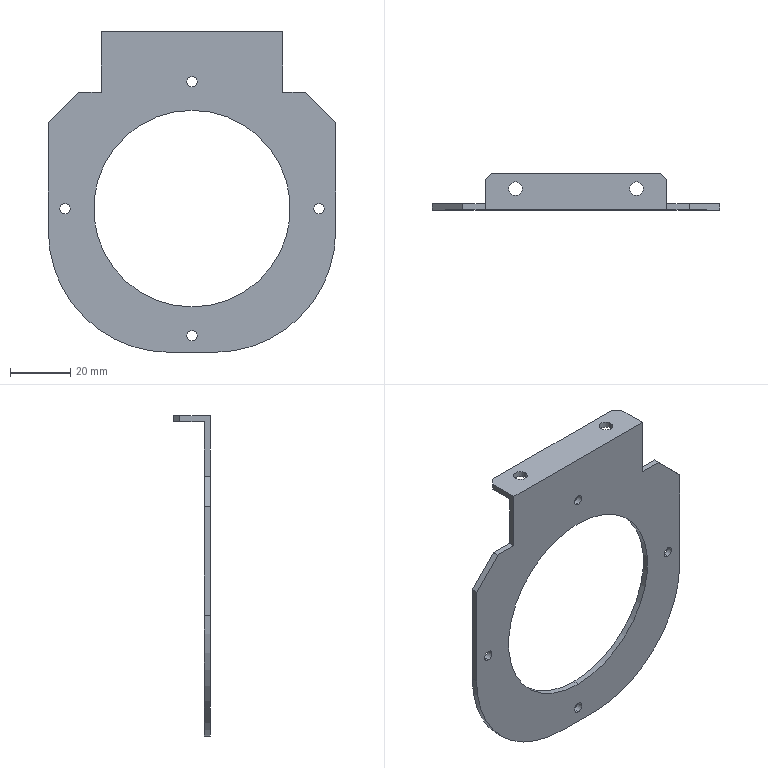Part | STEP file | PN_0021 | 1 solid | 32 faces | box 95 x 12 x 106 mm | volume 11586 mm3 | cylinder 16 | plane 16 | commonest cylinder face diameters 3.4 x8 4.5 x4 65 x2 80 x2